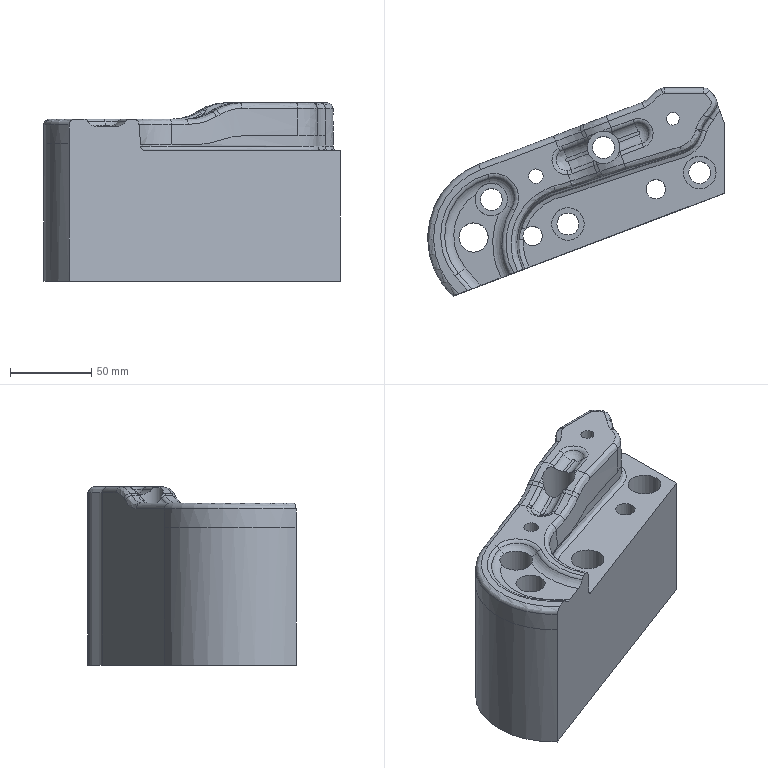Part | NX | features 23 2 | 1 solid | 107 faces | box 182.118 x 127.882 x 109.5 mm | volume 1066857 mm3 | cylinder 36 | spline 32 | torus 21 | plane 18 | commonest cylinder face diameters 7 x5 6 x4 13 x4 13.5 x4 20 x4 10 x2